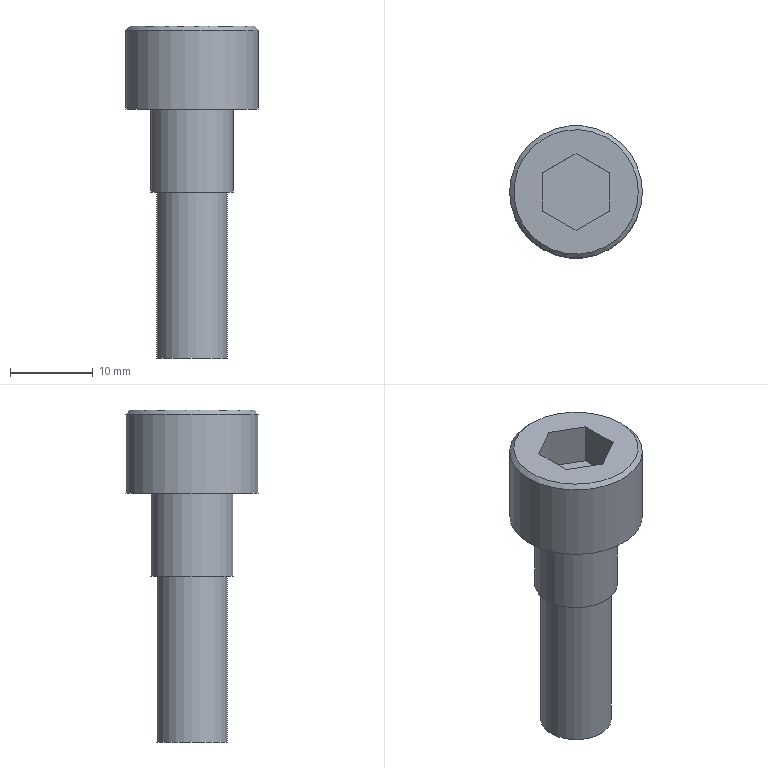Part | STEP file | M6-40_id1082_x_t | 1 solid | 15 faces | box 16 x 16 x 40 mm | volume 3648 mm3 | plane 11 | cylinder 3 | cone 1 | commonest cylinder face diameters 8.5 x1 10 x1 16 x1
STEP:
#1=CARTESIAN_POINT('',(-303.25,-147.5,-2.));
#2=VERTEX_POINT('',#1);
#3=CARTESIAN_POINT('',(-299.,-147.5,-2.));
#4=DIRECTION('',(0.,0.,-1.));
#5=DIRECTION('',(-1.,0.,0.));
#6=AXIS2_PLACEMENT_3D('',#3,#4,#5);
#7=CIRCLE('',#6,4.25);
#8=EDGE_CURVE('',#2,#2,#7,.T.);
#9=ORIENTED_EDGE('',*,*,#8,.F.);
#10=EDGE_LOOP('',(#9));
#11=FACE_BOUND('',#10,.T.);
#12=CARTESIAN_POINT('',(-294.,-147.5,-2.));
#13=VERTEX_POINT('',#12);
#14=CARTESIAN_POINT('',(-299.,-147.5,-2.));
#15=DIRECTION('',(0.,0.,1.));
#16=DIRECTION('',(1.,0.,0.));
#17=AXIS2_PLACEMENT_3D('',#14,#15,#16);
#18=CIRCLE('',#17,5.);
#19=EDGE_CURVE('',#13,#13,#18,.T.);
#20=ORIENTED_EDGE('',*,*,#19,.F.);
#21=EDGE_LOOP('',(#20));
#22=FACE_BOUND('',#21,.T.);
#23=CARTESIAN_POINT('',(-299.,-147.5,-2.));
#24=DIRECTION('',(0.,0.,-1.));
#25=DIRECTION('',(-1.,0.,0.));
#26=AXIS2_PLACEMENT_3D('',#23,#24,#25);
#27=PLANE('',#26);
#28=ADVANCED_FACE('',(#11,#22),#27,.T.);
#29=CARTESIAN_POINT('',(-304.,-147.5,8.));
#30=VERTEX_POINT('',#29);
#31=CARTESIAN_POINT('',(-299.,-147.5,8.));
#32=DIRECTION('',(0.,0.,1.));
#33=DIRECTION('',(-1.,0.,0.));
#34=AXIS2_PLACEMENT_3D('',#31,#32,#33);
#35=CIRCLE('',#34,5.);
#36=EDGE_CURVE('',#30,#30,#35,.T.);
#37=ORIENTED_EDGE('',*,*,#36,.F.);
#38=EDGE_LOOP('',(#37));
#39=FACE_BOUND('',#38,.T.);
#40=ORIENTED_EDGE('',*,*,#19,.T.);
#41=EDGE_LOOP('',(#40));
#42=FACE_BOUND('',#41,.T.);
#43=CARTESIAN_POINT('',(-299.,-147.5,-2.));
#44=DIRECTION('',(0.,0.,1.));
#45=DIRECTION('',(1.,0.,0.));
#46=AXIS2_PLACEMENT_3D('',#43,#44,#45);
#47=CYLINDRICAL_SURFACE('',#46,5.);
#48=ADVANCED_FACE('',(#39,#42),#47,.T.);
#49=CARTESIAN_POINT('',(-291.5,-147.5,18.));
#50=VERTEX_POINT('',#49);
#51=CARTESIAN_POINT('',(-299.,-147.5,18.));
#52=DIRECTION('',(0.,0.,1.));
#53=DIRECTION('',(1.,0.,0.));
#54=AXIS2_PLACEMENT_3D('',#51,#52,#53);
#55=CIRCLE('',#54,7.5);
#56=EDGE_CURVE('',#50,#50,#55,.T.);
#57=ORIENTED_EDGE('',*,*,#56,.T.);
#58=EDGE_LOOP('',(#57));
#59=FACE_BOUND('',#58,.T.);
#60=CARTESIAN_POINT('',(-303.,-145.191,18.));
#61=VERTEX_POINT('',#60);
#62=CARTESIAN_POINT('',(-303.,-149.809,18.));
#63=VERTEX_POINT('',#62);
#64=CARTESIAN_POINT('',(-303.,-145.191,18.));
#65=DIRECTION('',(0.,-1.,0.));
#66=VECTOR('',#65,1.);
#67=LINE('',#64,#66);
#68=EDGE_CURVE('',#61,#63,#67,.T.);
#69=ORIENTED_EDGE('',*,*,#68,.F.);
#70=CARTESIAN_POINT('',(-299.,-142.881,18.));
#71=VERTEX_POINT('',#70);
#72=CARTESIAN_POINT('',(-299.,-142.881,18.));
#73=DIRECTION('',(-0.866,-0.5,0.));
#74=VECTOR('',#73,1.);
#75=LINE('',#72,#74);
#76=EDGE_CURVE('',#71,#61,#75,.T.);
#77=ORIENTED_EDGE('',*,*,#76,.F.);
#78=CARTESIAN_POINT('',(-295.,-145.191,18.));
#79=VERTEX_POINT('',#78);
#80=CARTESIAN_POINT('',(-295.,-145.191,18.));
#81=DIRECTION('',(-0.866,0.5,0.));
#82=VECTOR('',#81,1.);
#83=LINE('',#80,#82);
#84=EDGE_CURVE('',#79,#71,#83,.T.);
#85=ORIENTED_EDGE('',*,*,#84,.F.);
#86=CARTESIAN_POINT('',(-295.,-149.809,18.));
#87=VERTEX_POINT('',#86);
#88=CARTESIAN_POINT('',(-295.,-149.809,18.));
#89=DIRECTION('',(0.,1.,0.));
#90=VECTOR('',#89,1.);
#91=LINE('',#88,#90);
#92=EDGE_CURVE('',#87,#79,#91,.T.);
#93=ORIENTED_EDGE('',*,*,#92,.F.);
#94=CARTESIAN_POINT('',(-299.,-152.119,18.));
#95=VERTEX_POINT('',#94);
#96=CARTESIAN_POINT('',(-299.,-152.119,18.));
#97=DIRECTION('',(0.866,0.5,0.));
#98=VECTOR('',#97,1.);
#99=LINE('',#96,#98);
#100=EDGE_CURVE('',#95,#87,#99,.T.);
#101=ORIENTED_EDGE('',*,*,#100,.F.);
#102=CARTESIAN_POINT('',(-303.,-149.809,18.));
#103=DIRECTION('',(0.866,-0.5,0.));
#104=VECTOR('',#103,1.);
#105=LINE('',#102,#104);
#106=EDGE_CURVE('',#63,#95,#105,.T.);
#107=ORIENTED_EDGE('',*,*,#106,.F.);
#108=EDGE_LOOP('',(#69,#77,#85,#93,#101,#107));
#109=FACE_BOUND('',#108,.T.);
#110=CARTESIAN_POINT('',(-299.,-147.5,18.));
#111=DIRECTION('',(0.,0.,1.));
#112=DIRECTION('',(1.,0.,0.));
#113=AXIS2_PLACEMENT_3D('',#110,#111,#112);
#114=PLANE('',#113);
#115=ADVANCED_FACE('',(#59,#109),#114,.T.);
#116=ORIENTED_EDGE('',*,*,#36,.T.);
#117=EDGE_LOOP('',(#116));
#118=FACE_BOUND('',#117,.T.);
#119=CARTESIAN_POINT('',(-291.,-147.5,8.));
#120=VERTEX_POINT('',#119);
#121=CARTESIAN_POINT('',(-299.,-147.5,8.));
#122=DIRECTION('',(0.,0.,1.));
#123=DIRECTION('',(1.,0.,0.));
#124=AXIS2_PLACEMENT_3D('',#121,#122,#123);
#125=CIRCLE('',#124,8.);
#126=EDGE_CURVE('',#120,#120,#125,.T.);
#127=ORIENTED_EDGE('',*,*,#126,.F.);
#128=EDGE_LOOP('',(#127));
#129=FACE_BOUND('',#128,.T.);
#130=CARTESIAN_POINT('',(-299.,-147.5,8.));
#131=DIRECTION('',(0.,0.,-1.));
#132=DIRECTION('',(-1.,0.,0.));
#133=AXIS2_PLACEMENT_3D('',#130,#131,#132);
#134=PLANE('',#133);
#135=ADVANCED_FACE('',(#118,#129),#134,.T.);
#136=CARTESIAN_POINT('',(-291.,-147.5,17.5));
#137=VERTEX_POINT('',#136);
#138=CARTESIAN_POINT('',(-299.,-147.5,17.5));
#139=DIRECTION('',(0.,0.,-1.));
#140=DIRECTION('',(1.,0.,0.));
#141=AXIS2_PLACEMENT_3D('',#138,#139,#140);
#142=CIRCLE('',#141,8.);
#143=EDGE_CURVE('',#137,#137,#142,.T.);
#144=ORIENTED_EDGE('',*,*,#143,.T.);
#145=EDGE_LOOP('',(#144));
#146=FACE_BOUND('',#145,.T.);
#147=ORIENTED_EDGE('',*,*,#126,.T.);
#148=EDGE_LOOP('',(#147));
#149=FACE_BOUND('',#148,.T.);
#150=CARTESIAN_POINT('',(-299.,-147.5,8.));
#151=DIRECTION('',(0.,0.,1.));
#152=DIRECTION('',(1.,0.,0.));
#153=AXIS2_PLACEMENT_3D('',#150,#151,#152);
#154=CYLINDRICAL_SURFACE('',#153,8.);
#155=ADVANCED_FACE('',(#146,#149),#154,.T.);
#156=CARTESIAN_POINT('',(-294.75,-147.5,-22.));
#157=VERTEX_POINT('',#156);
#158=CARTESIAN_POINT('',(-299.,-147.5,-22.));
#159=DIRECTION('',(0.,0.,1.));
#160=DIRECTION('',(1.,0.,0.));
#161=AXIS2_PLACEMENT_3D('',#158,#159,#160);
#162=CIRCLE('',#161,4.25);
#163=EDGE_CURVE('',#157,#157,#162,.T.);
#164=ORIENTED_EDGE('',*,*,#163,.F.);
#165=EDGE_LOOP('',(#164));
#166=FACE_OUTER_BOUND('',#165,.T.);
#167=CARTESIAN_POINT('',(-299.,-147.5,-22.));
#168=DIRECTION('',(0.,0.,-1.));
#169=DIRECTION('',(-1.,0.,0.));
#170=AXIS2_PLACEMENT_3D('',#167,#168,#169);
#171=PLANE('',#170);
#172=ADVANCED_FACE('',(#166),#171,.T.);
#173=ORIENTED_EDGE('',*,*,#163,.T.);
#174=EDGE_LOOP('',(#173));
#175=FACE_BOUND('',#174,.T.);
#176=ORIENTED_EDGE('',*,*,#8,.T.);
#177=EDGE_LOOP('',(#176));
#178=FACE_BOUND('',#177,.T.);
#179=CARTESIAN_POINT('',(-299.,-147.5,-2.));
#180=DIRECTION('',(0.,0.,-1.));
#181=DIRECTION('',(1.,0.,0.));
#182=AXIS2_PLACEMENT_3D('',#179,#180,#181);
#183=CYLINDRICAL_SURFACE('',#182,4.25);
#184=ADVANCED_FACE('',(#175,#178),#183,.T.);
#185=ORIENTED_EDGE('',*,*,#68,.T.);
#186=CARTESIAN_POINT('',(-303.,-149.809,13.));
#187=VERTEX_POINT('',#186);
#188=CARTESIAN_POINT('',(-303.,-149.809,13.));
#189=DIRECTION('',(0.,0.,-1.));
#190=VECTOR('',#189,1.);
#191=LINE('',#188,#190);
#192=EDGE_CURVE('',#63,#187,#191,.T.);
#193=ORIENTED_EDGE('',*,*,#192,.T.);
#194=CARTESIAN_POINT('',(-303.,-145.191,13.));
#195=VERTEX_POINT('',#194);
#196=CARTESIAN_POINT('',(-303.,-145.191,13.));
#197=DIRECTION('',(0.,1.,0.));
#198=VECTOR('',#197,1.);
#199=LINE('',#196,#198);
#200=EDGE_CURVE('',#187,#195,#199,.T.);
#201=ORIENTED_EDGE('',*,*,#200,.T.);
#202=CARTESIAN_POINT('',(-303.,-145.191,13.));
#203=DIRECTION('',(0.,0.,-1.));
#204=VECTOR('',#203,1.);
#205=LINE('',#202,#204);
#206=EDGE_CURVE('',#61,#195,#205,.T.);
#207=ORIENTED_EDGE('',*,*,#206,.F.);
#208=EDGE_LOOP('',(#185,#193,#201,#207));
#209=FACE_OUTER_BOUND('',#208,.T.);
#210=CARTESIAN_POINT('',(-303.,-145.191,13.));
#211=DIRECTION('',(-1.,0.,0.));
#212=DIRECTION('',(0.,-1.,0.));
#213=AXIS2_PLACEMENT_3D('',#210,#211,#212);
#214=PLANE('',#213);
#215=ADVANCED_FACE('',(#209),#214,.F.);
#216=ORIENTED_EDGE('',*,*,#106,.T.);
#217=CARTESIAN_POINT('',(-299.,-152.119,13.));
#218=VERTEX_POINT('',#217);
#219=CARTESIAN_POINT('',(-299.,-152.119,13.));
#220=DIRECTION('',(0.,0.,-1.));
#221=VECTOR('',#220,1.);
#222=LINE('',#219,#221);
#223=EDGE_CURVE('',#95,#218,#222,.T.);
#224=ORIENTED_EDGE('',*,*,#223,.T.);
#225=CARTESIAN_POINT('',(-303.,-149.809,13.));
#226=DIRECTION('',(-0.866,0.5,0.));
#227=VECTOR('',#226,1.);
#228=LINE('',#225,#227);
#229=EDGE_CURVE('',#218,#187,#228,.T.);
#230=ORIENTED_EDGE('',*,*,#229,.T.);
#231=ORIENTED_EDGE('',*,*,#192,.F.);
#232=EDGE_LOOP('',(#216,#224,#230,#231));
#233=FACE_OUTER_BOUND('',#232,.T.);
#234=CARTESIAN_POINT('',(-303.,-149.809,13.));
#235=DIRECTION('',(-0.5,-0.866,0.));
#236=DIRECTION('',(0.866,-0.5,0.));
#237=AXIS2_PLACEMENT_3D('',#234,#235,#236);
#238=PLANE('',#237);
#239=ADVANCED_FACE('',(#233),#238,.F.);
#240=ORIENTED_EDGE('',*,*,#100,.T.);
#241=CARTESIAN_POINT('',(-295.,-149.809,13.));
#242=VERTEX_POINT('',#241);
#243=CARTESIAN_POINT('',(-295.,-149.809,13.));
#244=DIRECTION('',(0.,0.,-1.));
#245=VECTOR('',#244,1.);
#246=LINE('',#243,#245);
#247=EDGE_CURVE('',#87,#242,#246,.T.);
#248=ORIENTED_EDGE('',*,*,#247,.T.);
#249=CARTESIAN_POINT('',(-299.,-152.119,13.));
#250=DIRECTION('',(-0.866,-0.5,0.));
#251=VECTOR('',#250,1.);
#252=LINE('',#249,#251);
#253=EDGE_CURVE('',#242,#218,#252,.T.);
#254=ORIENTED_EDGE('',*,*,#253,.T.);
#255=ORIENTED_EDGE('',*,*,#223,.F.);
#256=EDGE_LOOP('',(#240,#248,#254,#255));
#257=FACE_OUTER_BOUND('',#256,.T.);
#258=CARTESIAN_POINT('',(-299.,-152.119,13.));
#259=DIRECTION('',(0.5,-0.866,0.));
#260=DIRECTION('',(0.866,0.5,0.));
#261=AXIS2_PLACEMENT_3D('',#258,#259,#260);
#262=PLANE('',#261);
#263=ADVANCED_FACE('',(#257),#262,.F.);
#264=ORIENTED_EDGE('',*,*,#92,.T.);
#265=CARTESIAN_POINT('',(-295.,-145.191,13.));
#266=VERTEX_POINT('',#265);
#267=CARTESIAN_POINT('',(-295.,-145.191,13.));
#268=DIRECTION('',(0.,0.,-1.));
#269=VECTOR('',#268,1.);
#270=LINE('',#267,#269);
#271=EDGE_CURVE('',#79,#266,#270,.T.);
#272=ORIENTED_EDGE('',*,*,#271,.T.);
#273=CARTESIAN_POINT('',(-295.,-149.809,13.));
#274=DIRECTION('',(0.,-1.,0.));
#275=VECTOR('',#274,1.);
#276=LINE('',#273,#275);
#277=EDGE_CURVE('',#266,#242,#276,.T.);
#278=ORIENTED_EDGE('',*,*,#277,.T.);
#279=ORIENTED_EDGE('',*,*,#247,.F.);
#280=EDGE_LOOP('',(#264,#272,#278,#279));
#281=FACE_OUTER_BOUND('',#280,.T.);
#282=CARTESIAN_POINT('',(-295.,-149.809,13.));
#283=DIRECTION('',(1.,0.,0.));
#284=DIRECTION('',(0.,1.,0.));
#285=AXIS2_PLACEMENT_3D('',#282,#283,#284);
#286=PLANE('',#285);
#287=ADVANCED_FACE('',(#281),#286,.F.);
#288=ORIENTED_EDGE('',*,*,#84,.T.);
#289=CARTESIAN_POINT('',(-299.,-142.881,13.));
#290=VERTEX_POINT('',#289);
#291=CARTESIAN_POINT('',(-299.,-142.881,13.));
#292=DIRECTION('',(0.,0.,-1.));
#293=VECTOR('',#292,1.);
#294=LINE('',#291,#293);
#295=EDGE_CURVE('',#71,#290,#294,.T.);
#296=ORIENTED_EDGE('',*,*,#295,.T.);
#297=CARTESIAN_POINT('',(-295.,-145.191,13.));
#298=DIRECTION('',(0.866,-0.5,0.));
#299=VECTOR('',#298,1.);
#300=LINE('',#297,#299);
#301=EDGE_CURVE('',#290,#266,#300,.T.);
#302=ORIENTED_EDGE('',*,*,#301,.T.);
#303=ORIENTED_EDGE('',*,*,#271,.F.);
#304=EDGE_LOOP('',(#288,#296,#302,#303));
#305=FACE_OUTER_BOUND('',#304,.T.);
#306=CARTESIAN_POINT('',(-295.,-145.191,13.));
#307=DIRECTION('',(0.5,0.866,0.));
#308=DIRECTION('',(-0.866,0.5,0.));
#309=AXIS2_PLACEMENT_3D('',#306,#307,#308);
#310=PLANE('',#309);
#311=ADVANCED_FACE('',(#305),#310,.F.);
#312=ORIENTED_EDGE('',*,*,#76,.T.);
#313=ORIENTED_EDGE('',*,*,#206,.T.);
#314=CARTESIAN_POINT('',(-299.,-142.881,13.));
#315=DIRECTION('',(0.866,0.5,0.));
#316=VECTOR('',#315,1.);
#317=LINE('',#314,#316);
#318=EDGE_CURVE('',#195,#290,#317,.T.);
#319=ORIENTED_EDGE('',*,*,#318,.T.);
#320=ORIENTED_EDGE('',*,*,#295,.F.);
#321=EDGE_LOOP('',(#312,#313,#319,#320));
#322=FACE_OUTER_BOUND('',#321,.T.);
#323=CARTESIAN_POINT('',(-299.,-142.881,13.));
#324=DIRECTION('',(-0.5,0.866,0.));
#325=DIRECTION('',(-0.866,-0.5,0.));
#326=AXIS2_PLACEMENT_3D('',#323,#324,#325);
#327=PLANE('',#326);
#328=ADVANCED_FACE('',(#322),#327,.F.);
#329=ORIENTED_EDGE('',*,*,#200,.F.);
#330=ORIENTED_EDGE('',*,*,#229,.F.);
#331=ORIENTED_EDGE('',*,*,#253,.F.);
#332=ORIENTED_EDGE('',*,*,#277,.F.);
#333=ORIENTED_EDGE('',*,*,#301,.F.);
#334=ORIENTED_EDGE('',*,*,#318,.F.);
#335=EDGE_LOOP('',(#329,#330,#331,#332,#333,#334));
#336=FACE_OUTER_BOUND('',#335,.T.);
#337=CARTESIAN_POINT('',(-299.,-147.5,13.));
#338=DIRECTION('',(0.,0.,1.));
#339=DIRECTION('',(1.,0.,0.));
#340=AXIS2_PLACEMENT_3D('',#337,#338,#339);
#341=PLANE('',#340);
#342=ADVANCED_FACE('',(#336),#341,.T.);
#343=ORIENTED_EDGE('',*,*,#56,.F.);
#344=EDGE_LOOP('',(#343));
#345=FACE_BOUND('',#344,.T.);
#346=ORIENTED_EDGE('',*,*,#143,.F.);
#347=EDGE_LOOP('',(#346));
#348=FACE_BOUND('',#347,.T.);
#349=CARTESIAN_POINT('',(-299.,-147.5,17.5));
#350=DIRECTION('',(0.,0.,-1.));
#351=DIRECTION('',(-1.,0.,0.));
#352=AXIS2_PLACEMENT_3D('',#349,#350,#351);
#353=CONICAL_SURFACE('',#352,8.,45.);
#354=ADVANCED_FACE('',(#345,#348),#353,.T.);
#355=CLOSED_SHELL('',(#28,#48,#115,#135,#155,#172,#184,#215,#239,#263,#287,#311,#328,#342,#354));
#356=MANIFOLD_SOLID_BREP('',#355);
#357=(LENGTH_UNIT()NAMED_UNIT(*)SI_UNIT(.MILLI.,.METRE.));
#358=UNCERTAINTY_MEASURE_WITH_UNIT(LENGTH_MEASURE(0.00002),#357,'','');
#359=(NAMED_UNIT(*)PLANE_ANGLE_UNIT()SI_UNIT($,.RADIAN.));
#360=PLANE_ANGLE_MEASURE_WITH_UNIT(PLANE_ANGLE_MEASURE(0.01745),#359);
#361=DIMENSIONAL_EXPONENTS(0.,0.,0.,0.,0.,0.,0.);
#362=(CONVERSION_BASED_UNIT('DEGREE',#360)NAMED_UNIT(#361)PLANE_ANGLE_UNIT());
#363=(NAMED_UNIT(*)SI_UNIT($,.STERADIAN.)SOLID_ANGLE_UNIT());
#364=(GEOMETRIC_REPRESENTATION_CONTEXT(3)GLOBAL_UNCERTAINTY_ASSIGNED_CONTEXT((#358))GLOBAL_UNIT_ASSIGNED_CONTEXT((#357,#362,#363))REPRESENTATION_CONTEXT('',''));
#365=ADVANCED_BREP_SHAPE_REPRESENTATION('',(#356),#364);